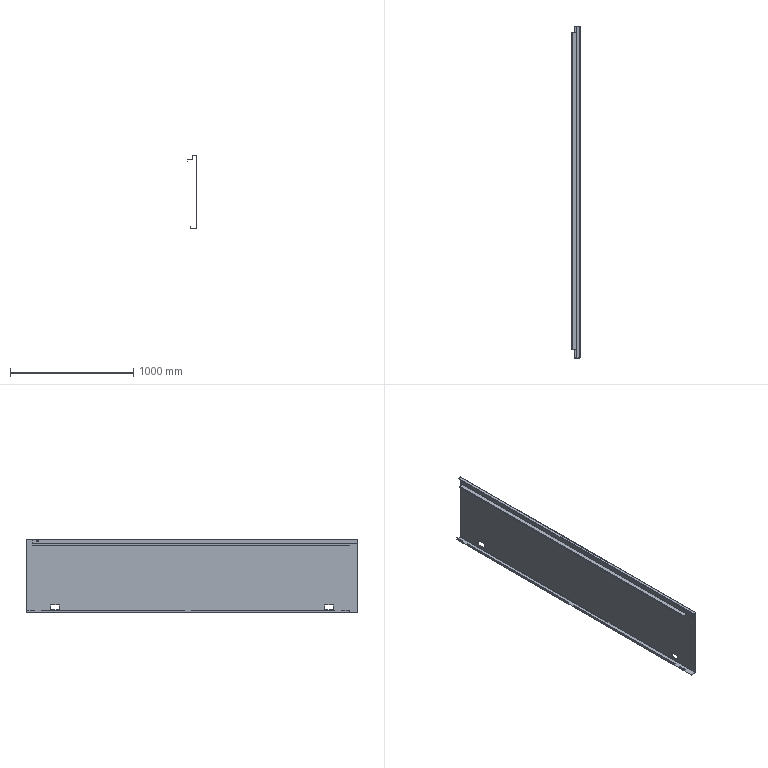Part | SolidWorks | features EdgeFlange 6, ICE 3, Fillet 1, FlatPattern 1, SMBaseFlange 1, SheetMetal 1 | 1 solid | 102 faces | box 68.5 x 2698 x 600 mm | volume 3118659 mm3 | plane 76 | cylinder 26 | commonest cylinder face diameters 6 x15 3 x9 10 x2